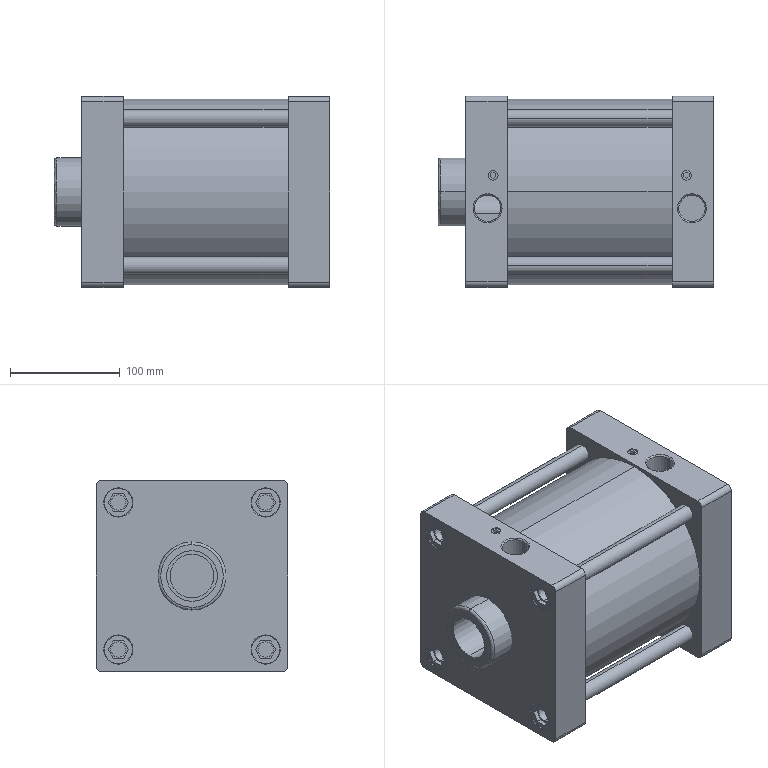Part | SolidWorks | features BaseBody 1 | 1 solid | 194 faces | box 251 x 174 x 174 mm | volume 2665389 mm3 | plane 106 | cylinder 66 | cone 20 | spline 2 | commonest cylinder face diameters 13.835 x16 25.6 x16 10 x8 16 x8 9 x4 24.117 x4